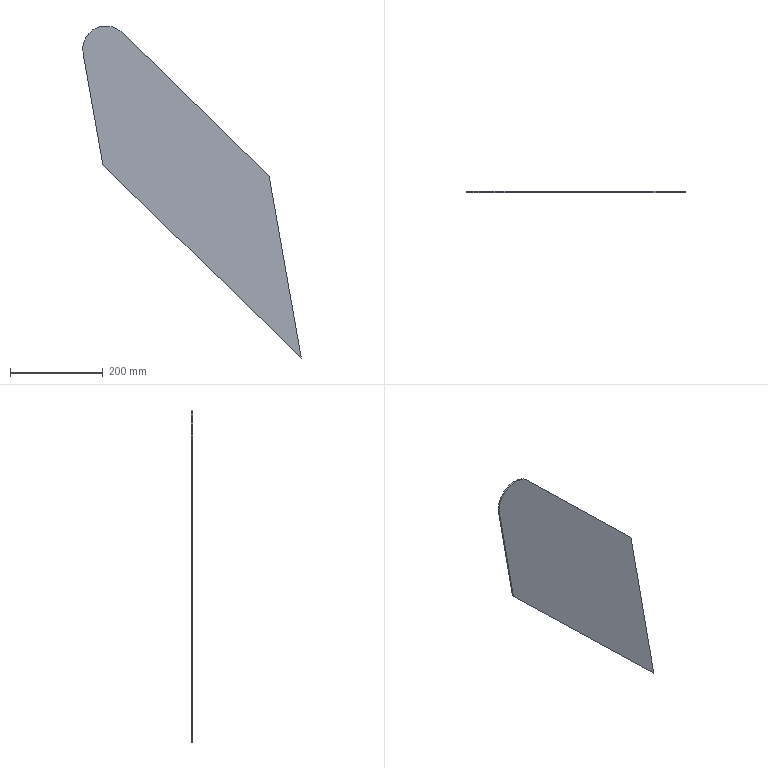Part | STEP file | floating channel side plate | 1 solid | 7 faces | box 471.639 x 3 x 716.945 mm | volume 405193 mm3 | plane 6 | cylinder 1 | commonest cylinder face diameters 100 x1
STEP:
#1=CARTESIAN_POINT('',(0.,0.,0.));
#2=DIRECTION('',(0.,0.,1.));
#3=DIRECTION('',(1.,0.,0.));
#4=AXIS2_PLACEMENT_3D('',#1,#2,#3);
#5=CARTESIAN_POINT('',(1599.684,308.,334.085));
#6=VERTEX_POINT('',#5);
#7=CARTESIAN_POINT('',(1683.806,308.,378.605));
#8=VERTEX_POINT('',#7);
#9=CARTESIAN_POINT('',(1648.922,308.,342.784));
#10=DIRECTION('',(0.,1.,0.));
#11=DIRECTION('',(0.,0.,1.));
#12=AXIS2_PLACEMENT_3D('',#9,#10,#11);
#13=CIRCLE('',#12,50.);
#14=CARTESIAN_POINT('',(1648.922,308.,342.784));
#15=DIRECTION('',(0.,-1.,0.));
#16=DIRECTION('',(0.,0.,1.));
#17=AXIS2_PLACEMENT_3D('',#14,#15,#16);
#18=CYLINDRICAL_SURFACE('',#17,50.);
#19=CARTESIAN_POINT('',(6.283,0.));
#20=DIRECTION('',(-1.,0.));
#21=VECTOR('',#20,1.);
#22=LINE('',#19,#21);
#23=(GEOMETRIC_REPRESENTATION_CONTEXT(2)PARAMETRIC_REPRESENTATION_CONTEXT()REPRESENTATION_CONTEXT('',''));
#24=DEFINITIONAL_REPRESENTATION('',(#22),#23);
#25=PCURVE('',#18,#24);
#26=CARTESIAN_POINT('',(0.,308.,0.));
#27=DIRECTION('',(0.,1.,0.));
#28=DIRECTION('',(0.,0.,-1.));
#29=AXIS2_PLACEMENT_3D('',#26,#27,#28);
#30=PLANE('',#29);
#31=CARTESIAN_POINT('',(-342.784,-1648.922));
#32=DIRECTION('',(-1.,0.));
#33=AXIS2_PLACEMENT_2D('',#31,#32);
#34=CIRCLE('',#33,50.);
#35=(GEOMETRIC_REPRESENTATION_CONTEXT(2)PARAMETRIC_REPRESENTATION_CONTEXT()REPRESENTATION_CONTEXT('',''));
#36=DEFINITIONAL_REPRESENTATION('',(#34),#35);
#37=PCURVE('',#30,#36);
#38=SURFACE_CURVE('',#13,(#25,#37),.PCURVE_S1.);
#39=EDGE_CURVE('',#6,#8,#38,.T.);
#40=ORIENTED_EDGE('',*,*,#39,.F.);
#41=CARTESIAN_POINT('',(1599.684,305.,334.085));
#42=VERTEX_POINT('',#41);
#43=CARTESIAN_POINT('',(1599.684,308.,334.085));
#44=DIRECTION('',(0.,1.,0.));
#45=VECTOR('',#44,1.);
#46=LINE('',#43,#45);
#47=CARTESIAN_POINT('',(1.746,0.));
#48=DIRECTION('',(0.,-1.));
#49=VECTOR('',#48,1.);
#50=LINE('',#47,#49);
#51=(GEOMETRIC_REPRESENTATION_CONTEXT(2)PARAMETRIC_REPRESENTATION_CONTEXT()REPRESENTATION_CONTEXT('',''));
#52=DEFINITIONAL_REPRESENTATION('',(#50),#51);
#53=PCURVE('',#18,#52);
#54=CARTESIAN_POINT('',(1642.295,308.,92.898));
#55=DIRECTION('',(0.9848,0.,0.174));
#56=DIRECTION('',(-0.174,0.,0.9848));
#57=AXIS2_PLACEMENT_3D('',#54,#55,#56);
#58=PLANE('',#57);
#59=CARTESIAN_POINT('',(244.922,0.));
#60=DIRECTION('',(0.,-1.));
#61=VECTOR('',#60,1.);
#62=LINE('',#59,#61);
#63=(GEOMETRIC_REPRESENTATION_CONTEXT(2)PARAMETRIC_REPRESENTATION_CONTEXT()REPRESENTATION_CONTEXT('',''));
#64=DEFINITIONAL_REPRESENTATION('',(#62),#63);
#65=PCURVE('',#58,#64);
#66=SURFACE_CURVE('',#46,(#53,#65),.PCURVE_S1.);
#67=EDGE_CURVE('',#42,#6,#66,.T.);
#68=ORIENTED_EDGE('',*,*,#67,.F.);
#69=CARTESIAN_POINT('',(1683.806,305.,378.605));
#70=VERTEX_POINT('',#69);
#71=CARTESIAN_POINT('',(1648.922,305.,342.784));
#72=DIRECTION('',(0.,-1.,0.));
#73=DIRECTION('',(0.,0.,1.));
#74=AXIS2_PLACEMENT_3D('',#71,#72,#73);
#75=CIRCLE('',#74,50.);
#76=CARTESIAN_POINT('',(-6.283,3.));
#77=DIRECTION('',(1.,0.));
#78=VECTOR('',#77,1.);
#79=LINE('',#76,#78);
#80=(GEOMETRIC_REPRESENTATION_CONTEXT(2)PARAMETRIC_REPRESENTATION_CONTEXT()REPRESENTATION_CONTEXT('',''));
#81=DEFINITIONAL_REPRESENTATION('',(#79),#80);
#82=PCURVE('',#18,#81);
#83=CARTESIAN_POINT('',(0.,305.,0.));
#84=DIRECTION('',(0.,1.,0.));
#85=DIRECTION('',(0.,0.,-1.));
#86=AXIS2_PLACEMENT_3D('',#83,#84,#85);
#87=PLANE('',#86);
#88=CARTESIAN_POINT('',(-392.784,-1648.922));
#89=CARTESIAN_POINT('',(-392.784,-1562.319));
#90=CARTESIAN_POINT('',(-317.784,-1605.621));
#91=CARTESIAN_POINT('',(-242.784,-1648.922));
#92=CARTESIAN_POINT('',(-317.784,-1692.223));
#93=CARTESIAN_POINT('',(-392.784,-1735.525));
#94=CARTESIAN_POINT('',(-392.784,-1648.922));
#95=(BOUNDED_CURVE()B_SPLINE_CURVE(2,(#88,#89,#90,#91,#92,#93,#94),.UNSPECIFIED.,.T.,.F.)B_SPLINE_CURVE_WITH_KNOTS((1,2,2,2,2,1),(-2.094,0.,2.094,4.189,6.283,8.378),.UNSPECIFIED.)CURVE()GEOMETRIC_REPRESENTATION_ITEM()RATIONAL_B_SPLINE_CURVE((1.,0.5,1.,0.5,1.,0.5,1.))REPRESENTATION_ITEM(''));
#96=(GEOMETRIC_REPRESENTATION_CONTEXT(2)PARAMETRIC_REPRESENTATION_CONTEXT()REPRESENTATION_CONTEXT('',''));
#97=DEFINITIONAL_REPRESENTATION('',(#95),#96);
#98=PCURVE('',#87,#97);
#99=SURFACE_CURVE('',#75,(#82,#98),.PCURVE_S1.);
#100=EDGE_CURVE('',#70,#42,#99,.T.);
#101=ORIENTED_EDGE('',*,*,#100,.F.);
#102=CARTESIAN_POINT('',(1683.806,308.,378.605));
#103=DIRECTION('',(0.,-1.,0.));
#104=VECTOR('',#103,1.);
#105=LINE('',#102,#104);
#106=CARTESIAN_POINT('',(-0.7721,0.));
#107=DIRECTION('',(0.,1.));
#108=VECTOR('',#107,1.);
#109=LINE('',#106,#108);
#110=(GEOMETRIC_REPRESENTATION_CONTEXT(2)PARAMETRIC_REPRESENTATION_CONTEXT()REPRESENTATION_CONTEXT('',''));
#111=DEFINITIONAL_REPRESENTATION('',(#109),#110);
#112=PCURVE('',#18,#111);
#113=CARTESIAN_POINT('',(1572.705,308.,486.798));
#114=DIRECTION('',(-0.6977,0.,-0.7164));
#115=DIRECTION('',(0.7164,0.,-0.6977));
#116=AXIS2_PLACEMENT_3D('',#113,#114,#115);
#117=PLANE('',#116);
#118=CARTESIAN_POINT('',(155.078,0.));
#119=DIRECTION('',(0.,1.));
#120=VECTOR('',#119,1.);
#121=LINE('',#118,#120);
#122=(GEOMETRIC_REPRESENTATION_CONTEXT(2)PARAMETRIC_REPRESENTATION_CONTEXT()REPRESENTATION_CONTEXT('',''));
#123=DEFINITIONAL_REPRESENTATION('',(#121),#122);
#124=PCURVE('',#117,#123);
#125=SURFACE_CURVE('',#105,(#112,#124),.PCURVE_S1.);
#126=EDGE_CURVE('',#8,#70,#125,.T.);
#127=ORIENTED_EDGE('',*,*,#126,.F.);
#128=EDGE_LOOP('',(#40,#68,#101,#127));
#129=FACE_BOUND('',#128,.T.);
#130=ADVANCED_FACE('',(#129),#18,.T.);
#131=CARTESIAN_POINT('',(2000.971,305.,69.739));
#132=VERTEX_POINT('',#131);
#133=CARTESIAN_POINT('',(1572.705,305.,486.798));
#134=DIRECTION('',(0.7164,0.,-0.6977));
#135=VECTOR('',#134,1.);
#136=LINE('',#133,#135);
#137=CARTESIAN_POINT('',(-486.798,-1572.705));
#138=DIRECTION('',(0.6977,-0.7164));
#139=VECTOR('',#138,1.);
#140=LINE('',#137,#139);
#141=(GEOMETRIC_REPRESENTATION_CONTEXT(2)PARAMETRIC_REPRESENTATION_CONTEXT()REPRESENTATION_CONTEXT('',''));
#142=DEFINITIONAL_REPRESENTATION('',(#140),#141);
#143=PCURVE('',#87,#142);
#144=CARTESIAN_POINT('',(0.,3.));
#145=DIRECTION('',(1.,0.));
#146=VECTOR('',#145,1.);
#147=LINE('',#144,#146);
#148=(GEOMETRIC_REPRESENTATION_CONTEXT(2)PARAMETRIC_REPRESENTATION_CONTEXT()REPRESENTATION_CONTEXT('',''));
#149=DEFINITIONAL_REPRESENTATION('',(#147),#148);
#150=PCURVE('',#117,#149);
#151=SURFACE_CURVE('',#136,(#143,#150),.PCURVE_S1.);
#152=EDGE_CURVE('',#70,#132,#151,.T.);
#153=ORIENTED_EDGE('',*,*,#152,.F.);
#154=ORIENTED_EDGE('',*,*,#100,.T.);
#155=CARTESIAN_POINT('',(1642.295,305.,92.898));
#156=VERTEX_POINT('',#155);
#157=CARTESIAN_POINT('',(1642.295,305.,92.898));
#158=DIRECTION('',(-0.174,0.,0.9848));
#159=VECTOR('',#158,1.);
#160=LINE('',#157,#159);
#161=CARTESIAN_POINT('',(-92.898,-1642.295));
#162=DIRECTION('',(-0.9848,0.174));
#163=VECTOR('',#162,1.);
#164=LINE('',#161,#163);
#165=(GEOMETRIC_REPRESENTATION_CONTEXT(2)PARAMETRIC_REPRESENTATION_CONTEXT()REPRESENTATION_CONTEXT('',''));
#166=DEFINITIONAL_REPRESENTATION('',(#164),#165);
#167=PCURVE('',#87,#166);
#168=CARTESIAN_POINT('',(0.,3.));
#169=DIRECTION('',(1.,0.));
#170=VECTOR('',#169,1.);
#171=LINE('',#168,#170);
#172=(GEOMETRIC_REPRESENTATION_CONTEXT(2)PARAMETRIC_REPRESENTATION_CONTEXT()REPRESENTATION_CONTEXT('',''));
#173=DEFINITIONAL_REPRESENTATION('',(#171),#172);
#174=PCURVE('',#58,#173);
#175=SURFACE_CURVE('',#160,(#167,#174),.PCURVE_S1.);
#176=EDGE_CURVE('',#156,#42,#175,.T.);
#177=ORIENTED_EDGE('',*,*,#176,.F.);
#178=CARTESIAN_POINT('',(2070.561,305.,-324.161));
#179=VERTEX_POINT('',#178);
#180=CARTESIAN_POINT('',(2070.561,305.,-324.161));
#181=DIRECTION('',(-0.7164,0.,0.6977));
#182=VECTOR('',#181,1.);
#183=LINE('',#180,#182);
#184=CARTESIAN_POINT('',(324.161,-2070.561));
#185=DIRECTION('',(-0.6977,0.7164));
#186=VECTOR('',#185,1.);
#187=LINE('',#184,#186);
#188=(GEOMETRIC_REPRESENTATION_CONTEXT(2)PARAMETRIC_REPRESENTATION_CONTEXT()REPRESENTATION_CONTEXT('',''));
#189=DEFINITIONAL_REPRESENTATION('',(#187),#188);
#190=PCURVE('',#87,#189);
#191=CARTESIAN_POINT('',(2070.561,308.,-324.161));
#192=DIRECTION('',(0.6977,0.,0.7164));
#193=DIRECTION('',(-0.7164,0.,0.6977));
#194=AXIS2_PLACEMENT_3D('',#191,#192,#193);
#195=PLANE('',#194);
#196=CARTESIAN_POINT('',(0.,3.));
#197=DIRECTION('',(1.,0.));
#198=VECTOR('',#197,1.);
#199=LINE('',#196,#198);
#200=(GEOMETRIC_REPRESENTATION_CONTEXT(2)PARAMETRIC_REPRESENTATION_CONTEXT()REPRESENTATION_CONTEXT('',''));
#201=DEFINITIONAL_REPRESENTATION('',(#199),#200);
#202=PCURVE('',#195,#201);
#203=SURFACE_CURVE('',#183,(#190,#202),.PCURVE_S1.);
#204=EDGE_CURVE('',#179,#156,#203,.T.);
#205=ORIENTED_EDGE('',*,*,#204,.F.);
#206=CARTESIAN_POINT('',(2000.971,305.,69.739));
#207=DIRECTION('',(0.174,0.,-0.9848));
#208=VECTOR('',#207,1.);
#209=LINE('',#206,#208);
#210=CARTESIAN_POINT('',(-69.739,-2000.971));
#211=DIRECTION('',(0.9848,-0.174));
#212=VECTOR('',#211,1.);
#213=LINE('',#210,#212);
#214=(GEOMETRIC_REPRESENTATION_CONTEXT(2)PARAMETRIC_REPRESENTATION_CONTEXT()REPRESENTATION_CONTEXT('',''));
#215=DEFINITIONAL_REPRESENTATION('',(#213),#214);
#216=PCURVE('',#87,#215);
#217=CARTESIAN_POINT('',(2000.971,308.,69.739));
#218=DIRECTION('',(-0.9848,0.,-0.174));
#219=DIRECTION('',(0.174,0.,-0.9848));
#220=AXIS2_PLACEMENT_3D('',#217,#218,#219);
#221=PLANE('',#220);
#222=CARTESIAN_POINT('',(0.,3.));
#223=DIRECTION('',(1.,0.));
#224=VECTOR('',#223,1.);
#225=LINE('',#222,#224);
#226=(GEOMETRIC_REPRESENTATION_CONTEXT(2)PARAMETRIC_REPRESENTATION_CONTEXT()REPRESENTATION_CONTEXT('',''));
#227=DEFINITIONAL_REPRESENTATION('',(#225),#226);
#228=PCURVE('',#221,#227);
#229=SURFACE_CURVE('',#209,(#216,#228),.PCURVE_S1.);
#230=EDGE_CURVE('',#132,#179,#229,.T.);
#231=ORIENTED_EDGE('',*,*,#230,.F.);
#232=EDGE_LOOP('',(#153,#154,#177,#205,#231));
#233=FACE_BOUND('',#232,.T.);
#234=ADVANCED_FACE('',(#233),#87,.F.);
#235=CARTESIAN_POINT('',(1642.295,308.,92.898));
#236=VERTEX_POINT('',#235);
#237=CARTESIAN_POINT('',(1642.295,308.,92.898));
#238=DIRECTION('',(-0.174,0.,0.9848));
#239=VECTOR('',#238,1.);
#240=LINE('',#237,#239);
#241=CARTESIAN_POINT('',(-92.898,-1642.295));
#242=DIRECTION('',(-0.9848,0.174));
#243=VECTOR('',#242,1.);
#244=LINE('',#241,#243);
#245=(GEOMETRIC_REPRESENTATION_CONTEXT(2)PARAMETRIC_REPRESENTATION_CONTEXT()REPRESENTATION_CONTEXT('',''));
#246=DEFINITIONAL_REPRESENTATION('',(#244),#245);
#247=PCURVE('',#30,#246);
#248=CARTESIAN_POINT('',(0.,0.));
#249=DIRECTION('',(1.,0.));
#250=VECTOR('',#249,1.);
#251=LINE('',#248,#250);
#252=(GEOMETRIC_REPRESENTATION_CONTEXT(2)PARAMETRIC_REPRESENTATION_CONTEXT()REPRESENTATION_CONTEXT('',''));
#253=DEFINITIONAL_REPRESENTATION('',(#251),#252);
#254=PCURVE('',#58,#253);
#255=SURFACE_CURVE('',#240,(#247,#254),.PCURVE_S1.);
#256=EDGE_CURVE('',#236,#6,#255,.T.);
#257=ORIENTED_EDGE('',*,*,#256,.T.);
#258=ORIENTED_EDGE('',*,*,#39,.T.);
#259=CARTESIAN_POINT('',(2000.971,308.,69.739));
#260=VERTEX_POINT('',#259);
#261=CARTESIAN_POINT('',(1572.705,308.,486.798));
#262=DIRECTION('',(0.7164,0.,-0.6977));
#263=VECTOR('',#262,1.);
#264=LINE('',#261,#263);
#265=CARTESIAN_POINT('',(-486.798,-1572.705));
#266=DIRECTION('',(0.6977,-0.7164));
#267=VECTOR('',#266,1.);
#268=LINE('',#265,#267);
#269=(GEOMETRIC_REPRESENTATION_CONTEXT(2)PARAMETRIC_REPRESENTATION_CONTEXT()REPRESENTATION_CONTEXT('',''));
#270=DEFINITIONAL_REPRESENTATION('',(#268),#269);
#271=PCURVE('',#30,#270);
#272=CARTESIAN_POINT('',(0.,0.));
#273=DIRECTION('',(1.,0.));
#274=VECTOR('',#273,1.);
#275=LINE('',#272,#274);
#276=(GEOMETRIC_REPRESENTATION_CONTEXT(2)PARAMETRIC_REPRESENTATION_CONTEXT()REPRESENTATION_CONTEXT('',''));
#277=DEFINITIONAL_REPRESENTATION('',(#275),#276);
#278=PCURVE('',#117,#277);
#279=SURFACE_CURVE('',#264,(#271,#278),.PCURVE_S1.);
#280=EDGE_CURVE('',#8,#260,#279,.T.);
#281=ORIENTED_EDGE('',*,*,#280,.T.);
#282=CARTESIAN_POINT('',(2070.561,308.,-324.161));
#283=VERTEX_POINT('',#282);
#284=CARTESIAN_POINT('',(2000.971,308.,69.739));
#285=DIRECTION('',(0.174,0.,-0.9848));
#286=VECTOR('',#285,1.);
#287=LINE('',#284,#286);
#288=CARTESIAN_POINT('',(-69.739,-2000.971));
#289=DIRECTION('',(0.9848,-0.174));
#290=VECTOR('',#289,1.);
#291=LINE('',#288,#290);
#292=(GEOMETRIC_REPRESENTATION_CONTEXT(2)PARAMETRIC_REPRESENTATION_CONTEXT()REPRESENTATION_CONTEXT('',''));
#293=DEFINITIONAL_REPRESENTATION('',(#291),#292);
#294=PCURVE('',#30,#293);
#295=CARTESIAN_POINT('',(0.,0.));
#296=DIRECTION('',(1.,0.));
#297=VECTOR('',#296,1.);
#298=LINE('',#295,#297);
#299=(GEOMETRIC_REPRESENTATION_CONTEXT(2)PARAMETRIC_REPRESENTATION_CONTEXT()REPRESENTATION_CONTEXT('',''));
#300=DEFINITIONAL_REPRESENTATION('',(#298),#299);
#301=PCURVE('',#221,#300);
#302=SURFACE_CURVE('',#287,(#294,#301),.PCURVE_S1.);
#303=EDGE_CURVE('',#260,#283,#302,.T.);
#304=ORIENTED_EDGE('',*,*,#303,.T.);
#305=CARTESIAN_POINT('',(2070.561,308.,-324.161));
#306=DIRECTION('',(-0.7164,0.,0.6977));
#307=VECTOR('',#306,1.);
#308=LINE('',#305,#307);
#309=CARTESIAN_POINT('',(324.161,-2070.561));
#310=DIRECTION('',(-0.6977,0.7164));
#311=VECTOR('',#310,1.);
#312=LINE('',#309,#311);
#313=(GEOMETRIC_REPRESENTATION_CONTEXT(2)PARAMETRIC_REPRESENTATION_CONTEXT()REPRESENTATION_CONTEXT('',''));
#314=DEFINITIONAL_REPRESENTATION('',(#312),#313);
#315=PCURVE('',#30,#314);
#316=CARTESIAN_POINT('',(0.,0.));
#317=DIRECTION('',(1.,0.));
#318=VECTOR('',#317,1.);
#319=LINE('',#316,#318);
#320=(GEOMETRIC_REPRESENTATION_CONTEXT(2)PARAMETRIC_REPRESENTATION_CONTEXT()REPRESENTATION_CONTEXT('',''));
#321=DEFINITIONAL_REPRESENTATION('',(#319),#320);
#322=PCURVE('',#195,#321);
#323=SURFACE_CURVE('',#308,(#315,#322),.PCURVE_S1.);
#324=EDGE_CURVE('',#283,#236,#323,.T.);
#325=ORIENTED_EDGE('',*,*,#324,.T.);
#326=EDGE_LOOP('',(#257,#258,#281,#304,#325));
#327=FACE_BOUND('',#326,.T.);
#328=ADVANCED_FACE('',(#327),#30,.T.);
#329=ORIENTED_EDGE('',*,*,#204,.T.);
#330=CARTESIAN_POINT('',(1642.295,308.,92.898));
#331=DIRECTION('',(0.,-1.,0.));
#332=VECTOR('',#331,1.);
#333=LINE('',#330,#332);
#334=CARTESIAN_POINT('',(597.788,0.));
#335=DIRECTION('',(0.,1.));
#336=VECTOR('',#335,1.);
#337=LINE('',#334,#336);
#338=(GEOMETRIC_REPRESENTATION_CONTEXT(2)PARAMETRIC_REPRESENTATION_CONTEXT()REPRESENTATION_CONTEXT('',''));
#339=DEFINITIONAL_REPRESENTATION('',(#337),#338);
#340=PCURVE('',#195,#339);
#341=CARTESIAN_POINT('',(0.,0.));
#342=DIRECTION('',(0.,1.));
#343=VECTOR('',#342,1.);
#344=LINE('',#341,#343);
#345=(GEOMETRIC_REPRESENTATION_CONTEXT(2)PARAMETRIC_REPRESENTATION_CONTEXT()REPRESENTATION_CONTEXT('',''));
#346=DEFINITIONAL_REPRESENTATION('',(#344),#345);
#347=PCURVE('',#58,#346);
#348=SURFACE_CURVE('',#333,(#340,#347),.PCURVE_S1.);
#349=EDGE_CURVE('',#236,#156,#348,.T.);
#350=ORIENTED_EDGE('',*,*,#349,.F.);
#351=ORIENTED_EDGE('',*,*,#324,.F.);
#352=CARTESIAN_POINT('',(2070.561,308.,-324.161));
#353=DIRECTION('',(0.,-1.,0.));
#354=VECTOR('',#353,1.);
#355=LINE('',#352,#354);
#356=CARTESIAN_POINT('',(0.,0.));
#357=DIRECTION('',(0.,1.));
#358=VECTOR('',#357,1.);
#359=LINE('',#356,#358);
#360=(GEOMETRIC_REPRESENTATION_CONTEXT(2)PARAMETRIC_REPRESENTATION_CONTEXT()REPRESENTATION_CONTEXT('',''));
#361=DEFINITIONAL_REPRESENTATION('',(#359),#360);
#362=PCURVE('',#195,#361);
#363=CARTESIAN_POINT('',(400.,0.));
#364=DIRECTION('',(0.,1.));
#365=VECTOR('',#364,1.);
#366=LINE('',#363,#365);
#367=(GEOMETRIC_REPRESENTATION_CONTEXT(2)PARAMETRIC_REPRESENTATION_CONTEXT()REPRESENTATION_CONTEXT('',''));
#368=DEFINITIONAL_REPRESENTATION('',(#366),#367);
#369=PCURVE('',#221,#368);
#370=SURFACE_CURVE('',#355,(#362,#369),.PCURVE_S1.);
#371=EDGE_CURVE('',#283,#179,#370,.T.);
#372=ORIENTED_EDGE('',*,*,#371,.T.);
#373=EDGE_LOOP('',(#329,#350,#351,#372));
#374=FACE_BOUND('',#373,.T.);
#375=ADVANCED_FACE('',(#374),#195,.F.);
#376=ORIENTED_EDGE('',*,*,#230,.T.);
#377=ORIENTED_EDGE('',*,*,#371,.F.);
#378=ORIENTED_EDGE('',*,*,#303,.F.);
#379=CARTESIAN_POINT('',(2000.971,308.,69.739));
#380=DIRECTION('',(0.,-1.,0.));
#381=VECTOR('',#380,1.);
#382=LINE('',#379,#381);
#383=CARTESIAN_POINT('',(0.,0.));
#384=DIRECTION('',(0.,1.));
#385=VECTOR('',#384,1.);
#386=LINE('',#383,#385);
#387=(GEOMETRIC_REPRESENTATION_CONTEXT(2)PARAMETRIC_REPRESENTATION_CONTEXT()REPRESENTATION_CONTEXT('',''));
#388=DEFINITIONAL_REPRESENTATION('',(#386),#387);
#389=PCURVE('',#221,#388);
#390=CARTESIAN_POINT('',(597.788,0.));
#391=DIRECTION('',(0.,1.));
#392=VECTOR('',#391,1.);
#393=LINE('',#390,#392);
#394=(GEOMETRIC_REPRESENTATION_CONTEXT(2)PARAMETRIC_REPRESENTATION_CONTEXT()REPRESENTATION_CONTEXT('',''));
#395=DEFINITIONAL_REPRESENTATION('',(#393),#394);
#396=PCURVE('',#117,#395);
#397=SURFACE_CURVE('',#382,(#389,#396),.PCURVE_S1.);
#398=EDGE_CURVE('',#260,#132,#397,.T.);
#399=ORIENTED_EDGE('',*,*,#398,.T.);
#400=EDGE_LOOP('',(#376,#377,#378,#399));
#401=FACE_BOUND('',#400,.T.);
#402=ADVANCED_FACE('',(#401),#221,.F.);
#403=ORIENTED_EDGE('',*,*,#280,.F.);
#404=ORIENTED_EDGE('',*,*,#126,.T.);
#405=ORIENTED_EDGE('',*,*,#152,.T.);
#406=ORIENTED_EDGE('',*,*,#398,.F.);
#407=EDGE_LOOP('',(#403,#404,#405,#406));
#408=FACE_BOUND('',#407,.T.);
#409=ADVANCED_FACE('',(#408),#117,.F.);
#410=ORIENTED_EDGE('',*,*,#176,.T.);
#411=ORIENTED_EDGE('',*,*,#67,.T.);
#412=ORIENTED_EDGE('',*,*,#256,.F.);
#413=ORIENTED_EDGE('',*,*,#349,.T.);
#414=EDGE_LOOP('',(#410,#411,#412,#413));
#415=FACE_BOUND('',#414,.T.);
#416=ADVANCED_FACE('',(#415),#58,.F.);
#417=CLOSED_SHELL('',(#130,#234,#328,#375,#402,#409,#416));
#418=MANIFOLD_SOLID_BREP('',#417);
#419=(LENGTH_UNIT()NAMED_UNIT(*)SI_UNIT(.MILLI.,.METRE.));
#420=UNCERTAINTY_MEASURE_WITH_UNIT(LENGTH_MEASURE(0.0000001),#419,'','');
#421=(NAMED_UNIT(*)PLANE_ANGLE_UNIT()SI_UNIT($,.RADIAN.));
#422=(NAMED_UNIT(*)SI_UNIT($,.STERADIAN.)SOLID_ANGLE_UNIT());
#423=(GEOMETRIC_REPRESENTATION_CONTEXT(3)GLOBAL_UNCERTAINTY_ASSIGNED_CONTEXT((#420))GLOBAL_UNIT_ASSIGNED_CONTEXT((#419,#421,#422))REPRESENTATION_CONTEXT('',''));
#424=ADVANCED_BREP_SHAPE_REPRESENTATION('',(#4,#418),#423);